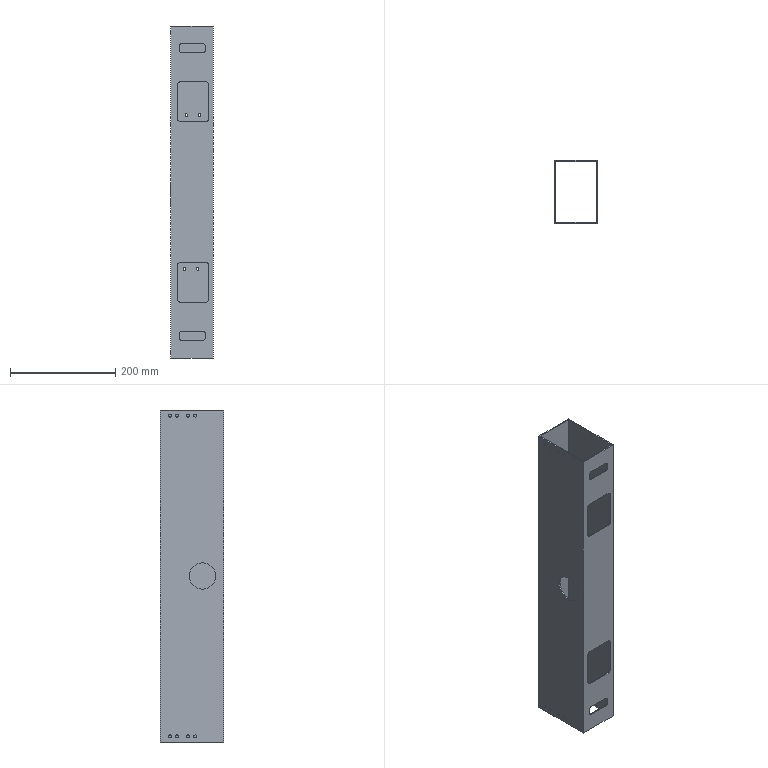Part | SolidWorks | features HoleWzd 2, Cut 1, ExtruThin 1, Fillet 1, ICE 1 | 1 solid | 76 faces | box 80 x 120 x 630 mm | volume 467928 mm3 | cylinder 50 | plane 26 | commonest cylinder face diameters 4.8 x16 5.8 x16 12 x16 50 x2